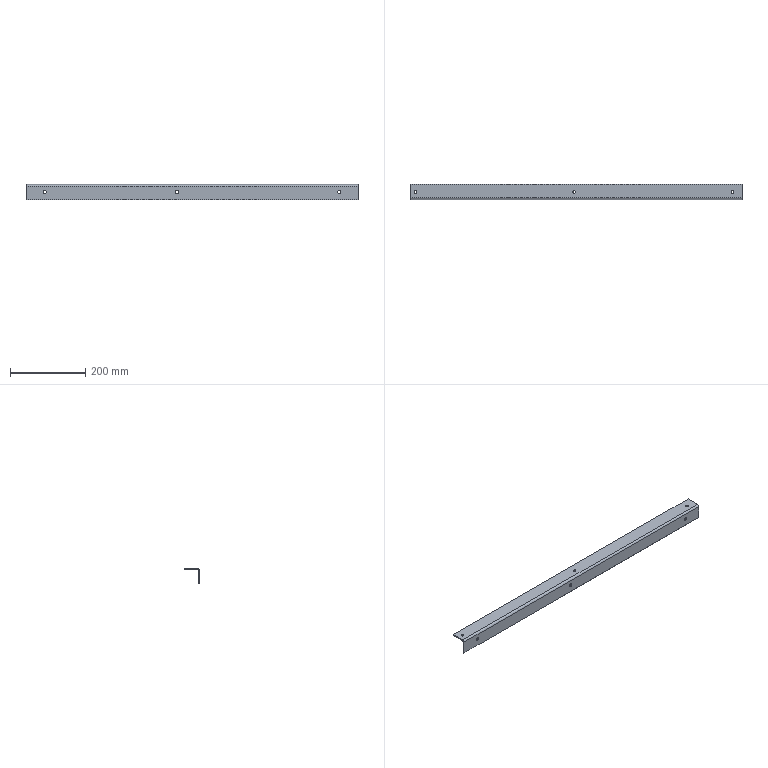Part | STEP file | 1 solid | 24 faces | box 880 x 40 x 40 mm | volume 196884 mm3 | cylinder 16 | plane 8 | commonest cylinder face diameters 7 x6 9 x6 4 x3 10 x1